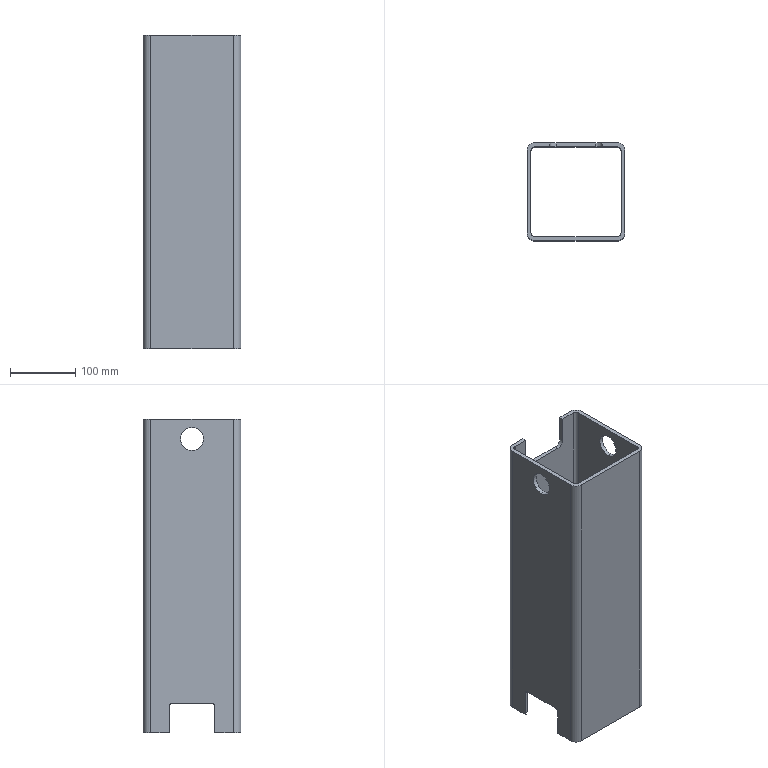Part | SolidWorks | features ICE 2, Attribute 1, Chamfer 1, Extrusion 1 | 1 solid | 48 faces | box 150 x 150 x 480 mm | volume 1538140 mm3 | plane 26 | cylinder 18 | cone 4 | commonest cylinder face diameters 10 x4 12 x4 24 x4 35 x4 20 x2
STEP:
#1=CARTESIAN_POINT('',(-75.,0.,227.5));
#2=VERTEX_POINT('',#1);
#3=CARTESIAN_POINT('',(-75.,0.,192.5));
#4=VERTEX_POINT('',#3);
#5=CARTESIAN_POINT('',(-75.,0.,210.));
#6=DIRECTION('',(1.,0.,0.));
#7=DIRECTION('',(0.,0.,-1.));
#8=AXIS2_PLACEMENT_3D('',#5,#6,#7);
#9=CIRCLE('',#8,17.5);
#10=EDGE_CURVE('',#2,#4,#9,.T.);
#11=ORIENTED_EDGE('',*,*,#10,.F.);
#12=CARTESIAN_POINT('',(-69.,0.,227.5));
#13=VERTEX_POINT('',#12);
#14=CARTESIAN_POINT('',(-75.,0.,227.5));
#15=DIRECTION('',(1.,0.,0.));
#16=VECTOR('',#15,1000.);
#17=LINE('',#14,#16);
#18=EDGE_CURVE('',#2,#13,#17,.T.);
#19=ORIENTED_EDGE('',*,*,#18,.T.);
#20=CARTESIAN_POINT('',(-69.,0.,192.5));
#21=VERTEX_POINT('',#20);
#22=CARTESIAN_POINT('',(-69.,0.,210.));
#23=DIRECTION('',(1.,0.,0.));
#24=DIRECTION('',(0.,0.,-1.));
#25=AXIS2_PLACEMENT_3D('',#22,#23,#24);
#26=CIRCLE('',#25,17.5);
#27=EDGE_CURVE('',#13,#21,#26,.T.);
#28=ORIENTED_EDGE('',*,*,#27,.T.);
#29=CARTESIAN_POINT('',(-75.,0.,192.5));
#30=DIRECTION('',(1.,0.,0.));
#31=VECTOR('',#30,1000.);
#32=LINE('',#29,#31);
#33=EDGE_CURVE('',#4,#21,#32,.T.);
#34=ORIENTED_EDGE('',*,*,#33,.F.);
#35=EDGE_LOOP('',(#11,#19,#28,#34));
#36=FACE_OUTER_BOUND('',#35,.T.);
#37=CARTESIAN_POINT('',(-75.,0.,210.));
#38=DIRECTION('',(1.,0.,0.));
#39=DIRECTION('',(0.,0.,-1.));
#40=AXIS2_PLACEMENT_3D('',#37,#38,#39);
#41=CYLINDRICAL_SURFACE('',#40,17.5);
#42=ADVANCED_FACE('',(#36),#41,.F.);
#43=CARTESIAN_POINT('',(69.,0.,192.5));
#44=VERTEX_POINT('',#43);
#45=CARTESIAN_POINT('',(69.,0.,227.5));
#46=VERTEX_POINT('',#45);
#47=CARTESIAN_POINT('',(69.,0.,210.));
#48=DIRECTION('',(-1.,0.,0.));
#49=DIRECTION('',(0.,0.,1.));
#50=AXIS2_PLACEMENT_3D('',#47,#48,#49);
#51=CIRCLE('',#50,17.5);
#52=EDGE_CURVE('',#44,#46,#51,.T.);
#53=ORIENTED_EDGE('',*,*,#52,.T.);
#54=CARTESIAN_POINT('',(75.,0.,227.5));
#55=VERTEX_POINT('',#54);
#56=CARTESIAN_POINT('',(-75.,0.,227.5));
#57=DIRECTION('',(1.,0.,0.));
#58=VECTOR('',#57,1000.);
#59=LINE('',#56,#58);
#60=EDGE_CURVE('',#46,#55,#59,.T.);
#61=ORIENTED_EDGE('',*,*,#60,.T.);
#62=CARTESIAN_POINT('',(75.,0.,192.5));
#63=VERTEX_POINT('',#62);
#64=CARTESIAN_POINT('',(75.,0.,210.));
#65=DIRECTION('',(1.,0.,0.));
#66=DIRECTION('',(0.,0.,-1.));
#67=AXIS2_PLACEMENT_3D('',#64,#65,#66);
#68=CIRCLE('',#67,17.5);
#69=EDGE_CURVE('',#55,#63,#68,.T.);
#70=ORIENTED_EDGE('',*,*,#69,.T.);
#71=CARTESIAN_POINT('',(-75.,0.,192.5));
#72=DIRECTION('',(1.,0.,0.));
#73=VECTOR('',#72,1000.);
#74=LINE('',#71,#73);
#75=EDGE_CURVE('',#44,#63,#74,.T.);
#76=ORIENTED_EDGE('',*,*,#75,.F.);
#77=EDGE_LOOP('',(#53,#61,#70,#76));
#78=FACE_OUTER_BOUND('',#77,.T.);
#79=CARTESIAN_POINT('',(-75.,0.,210.));
#80=DIRECTION('',(1.,0.,0.));
#81=DIRECTION('',(0.,0.,-1.));
#82=AXIS2_PLACEMENT_3D('',#79,#80,#81);
#83=CYLINDRICAL_SURFACE('',#82,17.5);
#84=ADVANCED_FACE('',(#78),#83,.F.);
#85=CARTESIAN_POINT('',(63.,-73.,-240.));
#86=VERTEX_POINT('',#85);
#87=CARTESIAN_POINT('',(73.,-63.,-240.));
#88=VERTEX_POINT('',#87);
#89=CARTESIAN_POINT('',(63.,-63.,-240.));
#90=DIRECTION('',(0.,0.,1.));
#91=DIRECTION('',(1.,0.,0.));
#92=AXIS2_PLACEMENT_3D('',#89,#90,#91);
#93=CIRCLE('',#92,10.);
#94=EDGE_CURVE('',#86,#88,#93,.T.);
#95=ORIENTED_EDGE('',*,*,#94,.T.);
#96=CARTESIAN_POINT('',(73.,-35.,-240.));
#97=VERTEX_POINT('',#96);
#98=CARTESIAN_POINT('',(73.,-35.,-240.));
#99=DIRECTION('',(0.,1.,0.));
#100=VECTOR('',#99,1000.);
#101=LINE('',#98,#100);
#102=EDGE_CURVE('',#88,#97,#101,.T.);
#103=ORIENTED_EDGE('',*,*,#102,.T.);
#104=CARTESIAN_POINT('',(75.,-35.,-240.));
#105=VERTEX_POINT('',#104);
#106=CARTESIAN_POINT('',(63.,-35.,-240.));
#107=DIRECTION('',(1.,0.,0.));
#108=VECTOR('',#107,1000.);
#109=LINE('',#106,#108);
#110=EDGE_CURVE('',#97,#105,#109,.T.);
#111=ORIENTED_EDGE('',*,*,#110,.T.);
#112=CARTESIAN_POINT('',(75.,-63.,-240.));
#113=VERTEX_POINT('',#112);
#114=CARTESIAN_POINT('',(75.,63.,-240.));
#115=DIRECTION('',(0.,1.,0.));
#116=VECTOR('',#115,1000.);
#117=LINE('',#114,#116);
#118=EDGE_CURVE('',#113,#105,#117,.T.);
#119=ORIENTED_EDGE('',*,*,#118,.F.);
#120=CARTESIAN_POINT('',(63.,-75.,-240.));
#121=VERTEX_POINT('',#120);
#122=CARTESIAN_POINT('',(63.,-63.,-240.));
#123=DIRECTION('',(0.,0.,1.));
#124=DIRECTION('',(1.,0.,0.));
#125=AXIS2_PLACEMENT_3D('',#122,#123,#124);
#126=CIRCLE('',#125,12.);
#127=EDGE_CURVE('',#121,#113,#126,.T.);
#128=ORIENTED_EDGE('',*,*,#127,.F.);
#129=CARTESIAN_POINT('',(-63.,-75.,-240.));
#130=VERTEX_POINT('',#129);
#131=CARTESIAN_POINT('',(-63.,-75.,-240.));
#132=DIRECTION('',(1.,0.,0.));
#133=VECTOR('',#132,1000.);
#134=LINE('',#131,#133);
#135=EDGE_CURVE('',#130,#121,#134,.T.);
#136=ORIENTED_EDGE('',*,*,#135,.F.);
#137=CARTESIAN_POINT('',(-75.,-63.,-240.));
#138=VERTEX_POINT('',#137);
#139=CARTESIAN_POINT('',(-63.,-63.,-240.));
#140=DIRECTION('',(0.,0.,1.));
#141=DIRECTION('',(1.,0.,0.));
#142=AXIS2_PLACEMENT_3D('',#139,#140,#141);
#143=CIRCLE('',#142,12.);
#144=EDGE_CURVE('',#138,#130,#143,.T.);
#145=ORIENTED_EDGE('',*,*,#144,.F.);
#146=CARTESIAN_POINT('',(-75.,-35.,-240.));
#147=VERTEX_POINT('',#146);
#148=CARTESIAN_POINT('',(-75.,-63.,-240.));
#149=DIRECTION('',(0.,-1.,0.));
#150=VECTOR('',#149,1000.);
#151=LINE('',#148,#150);
#152=EDGE_CURVE('',#147,#138,#151,.T.);
#153=ORIENTED_EDGE('',*,*,#152,.F.);
#154=CARTESIAN_POINT('',(-73.,-35.,-240.));
#155=VERTEX_POINT('',#154);
#156=CARTESIAN_POINT('',(63.,-35.,-240.));
#157=DIRECTION('',(1.,0.,0.));
#158=VECTOR('',#157,1000.);
#159=LINE('',#156,#158);
#160=EDGE_CURVE('',#147,#155,#159,.T.);
#161=ORIENTED_EDGE('',*,*,#160,.T.);
#162=CARTESIAN_POINT('',(-73.,-63.,-240.));
#163=VERTEX_POINT('',#162);
#164=CARTESIAN_POINT('',(-73.,-63.,-240.));
#165=DIRECTION('',(0.,-1.,0.));
#166=VECTOR('',#165,1000.);
#167=LINE('',#164,#166);
#168=EDGE_CURVE('',#155,#163,#167,.T.);
#169=ORIENTED_EDGE('',*,*,#168,.T.);
#170=CARTESIAN_POINT('',(-63.,-73.,-240.));
#171=VERTEX_POINT('',#170);
#172=CARTESIAN_POINT('',(-63.,-63.,-240.));
#173=DIRECTION('',(0.,0.,1.));
#174=DIRECTION('',(1.,0.,0.));
#175=AXIS2_PLACEMENT_3D('',#172,#173,#174);
#176=CIRCLE('',#175,10.);
#177=EDGE_CURVE('',#163,#171,#176,.T.);
#178=ORIENTED_EDGE('',*,*,#177,.T.);
#179=CARTESIAN_POINT('',(63.,-73.,-240.));
#180=DIRECTION('',(1.,0.,0.));
#181=VECTOR('',#180,1000.);
#182=LINE('',#179,#181);
#183=EDGE_CURVE('',#171,#86,#182,.T.);
#184=ORIENTED_EDGE('',*,*,#183,.T.);
#185=EDGE_LOOP('',(#95,#103,#111,#119,#128,#136,#145,#153,#161,#169,#178,#184));
#186=FACE_OUTER_BOUND('',#185,.T.);
#187=CARTESIAN_POINT('',(63.,63.,-240.));
#188=DIRECTION('',(0.,0.,1.));
#189=DIRECTION('',(1.,0.,0.));
#190=AXIS2_PLACEMENT_3D('',#187,#188,#189);
#191=PLANE('',#190);
#192=ADVANCED_FACE('',(#186),#191,.F.);
#193=CARTESIAN_POINT('',(63.,75.,240.));
#194=VERTEX_POINT('',#193);
#195=CARTESIAN_POINT('',(40.,75.,240.));
#196=VERTEX_POINT('',#195);
#197=CARTESIAN_POINT('',(63.,75.,240.));
#198=DIRECTION('',(-1.,0.,0.));
#199=VECTOR('',#198,1000.);
#200=LINE('',#197,#199);
#201=EDGE_CURVE('',#194,#196,#200,.T.);
#202=ORIENTED_EDGE('',*,*,#201,.T.);
#203=CARTESIAN_POINT('',(40.,69.,240.));
#204=VERTEX_POINT('',#203);
#205=CARTESIAN_POINT('',(40.,63.,240.));
#206=DIRECTION('',(0.,-1.,0.));
#207=VECTOR('',#206,1000.);
#208=LINE('',#205,#207);
#209=EDGE_CURVE('',#196,#204,#208,.T.);
#210=ORIENTED_EDGE('',*,*,#209,.T.);
#211=CARTESIAN_POINT('',(63.,69.,240.));
#212=VERTEX_POINT('',#211);
#213=CARTESIAN_POINT('',(63.,69.,240.));
#214=DIRECTION('',(-1.,0.,0.));
#215=VECTOR('',#214,1000.);
#216=LINE('',#213,#215);
#217=EDGE_CURVE('',#212,#204,#216,.T.);
#218=ORIENTED_EDGE('',*,*,#217,.F.);
#219=CARTESIAN_POINT('',(69.,63.,240.));
#220=VERTEX_POINT('',#219);
#221=CARTESIAN_POINT('',(63.,63.,240.));
#222=DIRECTION('',(0.,0.,1.));
#223=DIRECTION('',(1.,0.,0.));
#224=AXIS2_PLACEMENT_3D('',#221,#222,#223);
#225=CIRCLE('',#224,6.);
#226=EDGE_CURVE('',#220,#212,#225,.T.);
#227=ORIENTED_EDGE('',*,*,#226,.F.);
#228=CARTESIAN_POINT('',(69.,-63.,240.));
#229=VERTEX_POINT('',#228);
#230=CARTESIAN_POINT('',(69.,63.,240.));
#231=DIRECTION('',(0.,1.,0.));
#232=VECTOR('',#231,1000.);
#233=LINE('',#230,#232);
#234=EDGE_CURVE('',#229,#220,#233,.T.);
#235=ORIENTED_EDGE('',*,*,#234,.F.);
#236=CARTESIAN_POINT('',(63.,-69.,240.));
#237=VERTEX_POINT('',#236);
#238=CARTESIAN_POINT('',(63.,-63.,240.));
#239=DIRECTION('',(0.,0.,1.));
#240=DIRECTION('',(1.,0.,0.));
#241=AXIS2_PLACEMENT_3D('',#238,#239,#240);
#242=CIRCLE('',#241,6.);
#243=EDGE_CURVE('',#237,#229,#242,.T.);
#244=ORIENTED_EDGE('',*,*,#243,.F.);
#245=CARTESIAN_POINT('',(-63.,-69.,240.));
#246=VERTEX_POINT('',#245);
#247=CARTESIAN_POINT('',(-63.,-69.,240.));
#248=DIRECTION('',(1.,0.,0.));
#249=VECTOR('',#248,1000.);
#250=LINE('',#247,#249);
#251=EDGE_CURVE('',#246,#237,#250,.T.);
#252=ORIENTED_EDGE('',*,*,#251,.F.);
#253=CARTESIAN_POINT('',(-69.,-63.,240.));
#254=VERTEX_POINT('',#253);
#255=CARTESIAN_POINT('',(-63.,-63.,240.));
#256=DIRECTION('',(0.,0.,1.));
#257=DIRECTION('',(1.,0.,0.));
#258=AXIS2_PLACEMENT_3D('',#255,#256,#257);
#259=CIRCLE('',#258,6.);
#260=EDGE_CURVE('',#254,#246,#259,.T.);
#261=ORIENTED_EDGE('',*,*,#260,.F.);
#262=CARTESIAN_POINT('',(-69.,63.,240.));
#263=VERTEX_POINT('',#262);
#264=CARTESIAN_POINT('',(-69.,-63.,240.));
#265=DIRECTION('',(0.,-1.,0.));
#266=VECTOR('',#265,1000.);
#267=LINE('',#264,#266);
#268=EDGE_CURVE('',#263,#254,#267,.T.);
#269=ORIENTED_EDGE('',*,*,#268,.F.);
#270=CARTESIAN_POINT('',(-63.,69.,240.));
#271=VERTEX_POINT('',#270);
#272=CARTESIAN_POINT('',(-63.,63.,240.));
#273=DIRECTION('',(0.,0.,1.));
#274=DIRECTION('',(1.,0.,0.));
#275=AXIS2_PLACEMENT_3D('',#272,#273,#274);
#276=CIRCLE('',#275,6.);
#277=EDGE_CURVE('',#271,#263,#276,.T.);
#278=ORIENTED_EDGE('',*,*,#277,.F.);
#279=CARTESIAN_POINT('',(-40.,69.,240.));
#280=VERTEX_POINT('',#279);
#281=CARTESIAN_POINT('',(63.,69.,240.));
#282=DIRECTION('',(-1.,0.,0.));
#283=VECTOR('',#282,1000.);
#284=LINE('',#281,#283);
#285=EDGE_CURVE('',#280,#271,#284,.T.);
#286=ORIENTED_EDGE('',*,*,#285,.F.);
#287=CARTESIAN_POINT('',(-40.,75.,240.));
#288=VERTEX_POINT('',#287);
#289=CARTESIAN_POINT('',(-40.,63.,240.));
#290=DIRECTION('',(0.,1.,0.));
#291=VECTOR('',#290,1000.);
#292=LINE('',#289,#291);
#293=EDGE_CURVE('',#280,#288,#292,.T.);
#294=ORIENTED_EDGE('',*,*,#293,.T.);
#295=CARTESIAN_POINT('',(-63.,75.,240.));
#296=VERTEX_POINT('',#295);
#297=CARTESIAN_POINT('',(63.,75.,240.));
#298=DIRECTION('',(-1.,0.,0.));
#299=VECTOR('',#298,1000.);
#300=LINE('',#297,#299);
#301=EDGE_CURVE('',#288,#296,#300,.T.);
#302=ORIENTED_EDGE('',*,*,#301,.T.);
#303=CARTESIAN_POINT('',(-75.,63.,240.));
#304=VERTEX_POINT('',#303);
#305=CARTESIAN_POINT('',(-63.,63.,240.));
#306=DIRECTION('',(0.,0.,1.));
#307=DIRECTION('',(1.,0.,0.));
#308=AXIS2_PLACEMENT_3D('',#305,#306,#307);
#309=CIRCLE('',#308,12.);
#310=EDGE_CURVE('',#296,#304,#309,.T.);
#311=ORIENTED_EDGE('',*,*,#310,.T.);
#312=CARTESIAN_POINT('',(-75.,-63.,240.));
#313=VERTEX_POINT('',#312);
#314=CARTESIAN_POINT('',(-75.,-63.,240.));
#315=DIRECTION('',(0.,-1.,0.));
#316=VECTOR('',#315,1000.);
#317=LINE('',#314,#316);
#318=EDGE_CURVE('',#304,#313,#317,.T.);
#319=ORIENTED_EDGE('',*,*,#318,.T.);
#320=CARTESIAN_POINT('',(-63.,-75.,240.));
#321=VERTEX_POINT('',#320);
#322=CARTESIAN_POINT('',(-63.,-63.,240.));
#323=DIRECTION('',(0.,0.,1.));
#324=DIRECTION('',(1.,0.,0.));
#325=AXIS2_PLACEMENT_3D('',#322,#323,#324);
#326=CIRCLE('',#325,12.);
#327=EDGE_CURVE('',#313,#321,#326,.T.);
#328=ORIENTED_EDGE('',*,*,#327,.T.);
#329=CARTESIAN_POINT('',(63.,-75.,240.));
#330=VERTEX_POINT('',#329);
#331=CARTESIAN_POINT('',(-63.,-75.,240.));
#332=DIRECTION('',(1.,0.,0.));
#333=VECTOR('',#332,1000.);
#334=LINE('',#331,#333);
#335=EDGE_CURVE('',#321,#330,#334,.T.);
#336=ORIENTED_EDGE('',*,*,#335,.T.);
#337=CARTESIAN_POINT('',(75.,-63.,240.));
#338=VERTEX_POINT('',#337);
#339=CARTESIAN_POINT('',(63.,-63.,240.));
#340=DIRECTION('',(0.,0.,1.));
#341=DIRECTION('',(1.,0.,0.));
#342=AXIS2_PLACEMENT_3D('',#339,#340,#341);
#343=CIRCLE('',#342,12.);
#344=EDGE_CURVE('',#330,#338,#343,.T.);
#345=ORIENTED_EDGE('',*,*,#344,.T.);
#346=CARTESIAN_POINT('',(75.,63.,240.));
#347=VERTEX_POINT('',#346);
#348=CARTESIAN_POINT('',(75.,63.,240.));
#349=DIRECTION('',(0.,1.,0.));
#350=VECTOR('',#349,1000.);
#351=LINE('',#348,#350);
#352=EDGE_CURVE('',#338,#347,#351,.T.);
#353=ORIENTED_EDGE('',*,*,#352,.T.);
#354=CARTESIAN_POINT('',(63.,63.,240.));
#355=DIRECTION('',(0.,0.,1.));
#356=DIRECTION('',(1.,0.,0.));
#357=AXIS2_PLACEMENT_3D('',#354,#355,#356);
#358=CIRCLE('',#357,12.);
#359=EDGE_CURVE('',#347,#194,#358,.T.);
#360=ORIENTED_EDGE('',*,*,#359,.T.);
#361=EDGE_LOOP('',(#202,#210,#218,#227,#235,#244,#252,#261,#269,#278,#286,#294,#302,#311,#319,#328,#336,#345,#353,#360));
#362=FACE_OUTER_BOUND('',#361,.T.);
#363=CARTESIAN_POINT('',(63.,63.,240.));
#364=DIRECTION('',(0.,0.,1.));
#365=DIRECTION('',(1.,0.,0.));
#366=AXIS2_PLACEMENT_3D('',#363,#364,#365);
#367=PLANE('',#366);
#368=ADVANCED_FACE('',(#362),#367,.T.);
#369=CARTESIAN_POINT('',(40.,75.,200.));
#370=VERTEX_POINT('',#369);
#371=CARTESIAN_POINT('',(40.,75.,290.));
#372=DIRECTION('',(0.,0.,-1.));
#373=VECTOR('',#372,1000.);
#374=LINE('',#371,#373);
#375=EDGE_CURVE('',#196,#370,#374,.T.);
#376=ORIENTED_EDGE('',*,*,#375,.F.);
#377=ORIENTED_EDGE('',*,*,#201,.F.);
#378=CARTESIAN_POINT('',(63.,75.,-240.));
#379=VERTEX_POINT('',#378);
#380=CARTESIAN_POINT('',(63.,75.,240.));
#381=DIRECTION('',(0.,0.,-1.));
#382=VECTOR('',#381,1000.);
#383=LINE('',#380,#382);
#384=EDGE_CURVE('',#194,#379,#383,.T.);
#385=ORIENTED_EDGE('',*,*,#384,.T.);
#386=CARTESIAN_POINT('',(-63.,75.,-240.));
#387=VERTEX_POINT('',#386);
#388=CARTESIAN_POINT('',(63.,75.,-240.));
#389=DIRECTION('',(-1.,0.,0.));
#390=VECTOR('',#389,1000.);
#391=LINE('',#388,#390);
#392=EDGE_CURVE('',#379,#387,#391,.T.);
#393=ORIENTED_EDGE('',*,*,#392,.T.);
#394=CARTESIAN_POINT('',(-63.,75.,240.));
#395=DIRECTION('',(0.,0.,-1.));
#396=VECTOR('',#395,1000.);
#397=LINE('',#394,#396);
#398=EDGE_CURVE('',#296,#387,#397,.T.);
#399=ORIENTED_EDGE('',*,*,#398,.F.);
#400=ORIENTED_EDGE('',*,*,#301,.F.);
#401=CARTESIAN_POINT('',(-40.,75.,200.));
#402=VERTEX_POINT('',#401);
#403=CARTESIAN_POINT('',(-40.,75.,290.));
#404=DIRECTION('',(0.,0.,1.));
#405=VECTOR('',#404,1000.);
#406=LINE('',#403,#405);
#407=EDGE_CURVE('',#402,#288,#406,.T.);
#408=ORIENTED_EDGE('',*,*,#407,.F.);
#409=CARTESIAN_POINT('',(-30.,75.,190.));
#410=VERTEX_POINT('',#409);
#411=CARTESIAN_POINT('',(-30.,75.,200.));
#412=DIRECTION('',(0.,1.,0.));
#413=DIRECTION('',(0.,0.,1.));
#414=AXIS2_PLACEMENT_3D('',#411,#412,#413);
#415=CIRCLE('',#414,10.);
#416=EDGE_CURVE('',#410,#402,#415,.T.);
#417=ORIENTED_EDGE('',*,*,#416,.F.);
#418=CARTESIAN_POINT('',(30.,75.,190.));
#419=VERTEX_POINT('',#418);
#420=CARTESIAN_POINT('',(30.,75.,190.));
#421=DIRECTION('',(-1.,0.,0.));
#422=VECTOR('',#421,1000.);
#423=LINE('',#420,#422);
#424=EDGE_CURVE('',#419,#410,#423,.T.);
#425=ORIENTED_EDGE('',*,*,#424,.F.);
#426=CARTESIAN_POINT('',(30.,75.,200.));
#427=DIRECTION('',(0.,1.,0.));
#428=DIRECTION('',(0.,0.,1.));
#429=AXIS2_PLACEMENT_3D('',#426,#427,#428);
#430=CIRCLE('',#429,10.);
#431=EDGE_CURVE('',#370,#419,#430,.T.);
#432=ORIENTED_EDGE('',*,*,#431,.F.);
#433=EDGE_LOOP('',(#376,#377,#385,#393,#399,#400,#408,#417,#425,#432));
#434=FACE_OUTER_BOUND('',#433,.T.);
#435=CARTESIAN_POINT('',(63.,75.,240.));
#436=DIRECTION('',(0.,-1.,0.));
#437=DIRECTION('',(0.,0.,-1.));
#438=AXIS2_PLACEMENT_3D('',#435,#436,#437);
#439=PLANE('',#438);
#440=ADVANCED_FACE('',(#434),#439,.F.);
#441=CARTESIAN_POINT('',(-63.,69.,-236.));
#442=VERTEX_POINT('',#441);
#443=CARTESIAN_POINT('',(-63.,69.,240.));
#444=DIRECTION('',(0.,0.,-1.));
#445=VECTOR('',#444,1000.);
#446=LINE('',#443,#445);
#447=EDGE_CURVE('',#271,#442,#446,.T.);
#448=ORIENTED_EDGE('',*,*,#447,.T.);
#449=CARTESIAN_POINT('',(63.,69.,-236.));
#450=VERTEX_POINT('',#449);
#451=CARTESIAN_POINT('',(63.,69.,-236.));
#452=DIRECTION('',(1.,0.,0.));
#453=VECTOR('',#452,1000.);
#454=LINE('',#451,#453);
#455=EDGE_CURVE('',#442,#450,#454,.T.);
#456=ORIENTED_EDGE('',*,*,#455,.T.);
#457=CARTESIAN_POINT('',(63.,69.,240.));
#458=DIRECTION('',(0.,0.,-1.));
#459=VECTOR('',#458,1000.);
#460=LINE('',#457,#459);
#461=EDGE_CURVE('',#212,#450,#460,.T.);
#462=ORIENTED_EDGE('',*,*,#461,.F.);
#463=ORIENTED_EDGE('',*,*,#217,.T.);
#464=CARTESIAN_POINT('',(40.,69.,200.));
#465=VERTEX_POINT('',#464);
#466=CARTESIAN_POINT('',(40.,69.,240.));
#467=DIRECTION('',(0.,0.,-1.));
#468=VECTOR('',#467,1000.);
#469=LINE('',#466,#468);
#470=EDGE_CURVE('',#204,#465,#469,.T.);
#471=ORIENTED_EDGE('',*,*,#470,.T.);
#472=CARTESIAN_POINT('',(30.,69.,190.));
#473=VERTEX_POINT('',#472);
#474=CARTESIAN_POINT('',(30.,69.,200.));
#475=DIRECTION('',(0.,1.,0.));
#476=DIRECTION('',(0.,0.,-1.));
#477=AXIS2_PLACEMENT_3D('',#474,#475,#476);
#478=CIRCLE('',#477,10.);
#479=EDGE_CURVE('',#465,#473,#478,.T.);
#480=ORIENTED_EDGE('',*,*,#479,.T.);
#481=CARTESIAN_POINT('',(-30.,69.,190.));
#482=VERTEX_POINT('',#481);
#483=CARTESIAN_POINT('',(63.,69.,190.));
#484=DIRECTION('',(-1.,0.,0.));
#485=VECTOR('',#484,1000.);
#486=LINE('',#483,#485);
#487=EDGE_CURVE('',#473,#482,#486,.T.);
#488=ORIENTED_EDGE('',*,*,#487,.T.);
#489=CARTESIAN_POINT('',(-40.,69.,200.));
#490=VERTEX_POINT('',#489);
#491=CARTESIAN_POINT('',(-30.,69.,200.));
#492=DIRECTION('',(0.,1.,0.));
#493=DIRECTION('',(0.,0.,-1.));
#494=AXIS2_PLACEMENT_3D('',#491,#492,#493);
#495=CIRCLE('',#494,10.);
#496=EDGE_CURVE('',#482,#490,#495,.T.);
#497=ORIENTED_EDGE('',*,*,#496,.T.);
#498=CARTESIAN_POINT('',(-40.,69.,240.));
#499=DIRECTION('',(0.,0.,1.));
#500=VECTOR('',#499,1000.);
#501=LINE('',#498,#500);
#502=EDGE_CURVE('',#490,#280,#501,.T.);
#503=ORIENTED_EDGE('',*,*,#502,.T.);
#504=ORIENTED_EDGE('',*,*,#285,.T.);
#505=EDGE_LOOP('',(#448,#456,#462,#463,#471,#480,#488,#497,#503,#504));
#506=FACE_OUTER_BOUND('',#505,.T.);
#507=CARTESIAN_POINT('',(63.,69.,240.));
#508=DIRECTION('',(0.,-1.,0.));
#509=DIRECTION('',(0.,0.,-1.));
#510=AXIS2_PLACEMENT_3D('',#507,#508,#509);
#511=PLANE('',#510);
#512=ADVANCED_FACE('',(#506),#511,.T.);
#513=CARTESIAN_POINT('',(75.,35.,-240.));
#514=VERTEX_POINT('',#513);
#515=CARTESIAN_POINT('',(73.,35.,-240.));
#516=VERTEX_POINT('',#515);
#517=CARTESIAN_POINT('',(63.,35.,-240.));
#518=DIRECTION('',(-1.,0.,0.));
#519=VECTOR('',#518,1000.);
#520=LINE('',#517,#519);
#521=EDGE_CURVE('',#514,#516,#520,.T.);
#522=ORIENTED_EDGE('',*,*,#521,.T.);
#523=CARTESIAN_POINT('',(73.,63.,-240.));
#524=VERTEX_POINT('',#523);
#525=CARTESIAN_POINT('',(73.,63.,-240.));
#526=DIRECTION('',(0.,1.,0.));
#527=VECTOR('',#526,1000.);
#528=LINE('',#525,#527);
#529=EDGE_CURVE('',#516,#524,#528,.T.);
#530=ORIENTED_EDGE('',*,*,#529,.T.);
#531=CARTESIAN_POINT('',(63.,73.,-240.));
#532=VERTEX_POINT('',#531);
#533=CARTESIAN_POINT('',(63.,63.,-240.));
#534=DIRECTION('',(0.,0.,1.));
#535=DIRECTION('',(1.,0.,0.));
#536=AXIS2_PLACEMENT_3D('',#533,#534,#535);
#537=CIRCLE('',#536,10.);
#538=EDGE_CURVE('',#524,#532,#537,.T.);
#539=ORIENTED_EDGE('',*,*,#538,.T.);
#540=CARTESIAN_POINT('',(-63.,73.,-240.));
#541=VERTEX_POINT('',#540);
#542=CARTESIAN_POINT('',(-63.,73.,-240.));
#543=DIRECTION('',(-1.,0.,0.));
#544=VECTOR('',#543,1000.);
#545=LINE('',#542,#544);
#546=EDGE_CURVE('',#532,#541,#545,.T.);
#547=ORIENTED_EDGE('',*,*,#546,.T.);
#548=CARTESIAN_POINT('',(-73.,63.,-240.));
#549=VERTEX_POINT('',#548);
#550=CARTESIAN_POINT('',(-63.,63.,-240.));
#551=DIRECTION('',(0.,0.,1.));
#552=DIRECTION('',(1.,0.,0.));
#553=AXIS2_PLACEMENT_3D('',#550,#551,#552);
#554=CIRCLE('',#553,10.);
#555=EDGE_CURVE('',#541,#549,#554,.T.);
#556=ORIENTED_EDGE('',*,*,#555,.T.);
#557=CARTESIAN_POINT('',(-73.,35.,-240.));
#558=VERTEX_POINT('',#557);
#559=CARTESIAN_POINT('',(-73.,35.,-240.));
#560=DIRECTION('',(0.,-1.,0.));
#561=VECTOR('',#560,1000.);
#562=LINE('',#559,#561);
#563=EDGE_CURVE('',#549,#558,#562,.T.);
#564=ORIENTED_EDGE('',*,*,#563,.T.);
#565=CARTESIAN_POINT('',(-75.,35.,-240.));
#566=VERTEX_POINT('',#565);
#567=CARTESIAN_POINT('',(63.,35.,-240.));
#568=DIRECTION('',(-1.,0.,0.));
#569=VECTOR('',#568,1000.);
#570=LINE('',#567,#569);
#571=EDGE_CURVE('',#558,#566,#570,.T.);
#572=ORIENTED_EDGE('',*,*,#571,.T.);
#573=CARTESIAN_POINT('',(-75.,63.,-240.));
#574=VERTEX_POINT('',#573);
#575=CARTESIAN_POINT('',(-75.,-63.,-240.));
#576=DIRECTION('',(0.,-1.,0.));
#577=VECTOR('',#576,1000.);
#578=LINE('',#575,#577);
#579=EDGE_CURVE('',#574,#566,#578,.T.);
#580=ORIENTED_EDGE('',*,*,#579,.F.);
#581=CARTESIAN_POINT('',(-63.,63.,-240.));
#582=DIRECTION('',(0.,0.,1.));
#583=DIRECTION('',(1.,0.,0.));
#584=AXIS2_PLACEMENT_3D('',#581,#582,#583);
#585=CIRCLE('',#584,12.);
#586=EDGE_CURVE('',#387,#574,#585,.T.);
#587=ORIENTED_EDGE('',*,*,#586,.F.);
#588=ORIENTED_EDGE('',*,*,#392,.F.);
#589=CARTESIAN_POINT('',(75.,63.,-240.));
#590=VERTEX_POINT('',#589);
#591=CARTESIAN_POINT('',(63.,63.,-240.));
#592=DIRECTION('',(0.,0.,1.));
#593=DIRECTION('',(1.,0.,0.));
#594=AXIS2_PLACEMENT_3D('',#591,#592,#593);
#595=CIRCLE('',#594,12.);
#596=EDGE_CURVE('',#590,#379,#595,.T.);
#597=ORIENTED_EDGE('',*,*,#596,.F.);
#598=CARTESIAN_POINT('',(75.,63.,-240.));
#599=DIRECTION('',(0.,1.,0.));
#600=VECTOR('',#599,1000.);
#601=LINE('',#598,#600);
#602=EDGE_CURVE('',#514,#590,#601,.T.);
#603=ORIENTED_EDGE('',*,*,#602,.F.);
#604=EDGE_LOOP('',(#522,#530,#539,#547,#556,#564,#572,#580,#587,#588,#597,#603));
#605=FACE_OUTER_BOUND('',#604,.T.);
#606=CARTESIAN_POINT('',(63.,63.,-240.));
#607=DIRECTION('',(0.,0.,1.));
#608=DIRECTION('',(1.,0.,0.));
#609=AXIS2_PLACEMENT_3D('',#606,#607,#608);
#610=PLANE('',#609);
#611=ADVANCED_FACE('',(#605),#610,.F.);
#612=ORIENTED_EDGE('',*,*,#596,.T.);
#613=ORIENTED_EDGE('',*,*,#384,.F.);
#614=ORIENTED_EDGE('',*,*,#359,.F.);
#615=CARTESIAN_POINT('',(75.,63.,240.));
#616=DIRECTION('',(0.,0.,-1.));
#617=VECTOR('',#616,1000.);
#618=LINE('',#615,#617);
#619=EDGE_CURVE('',#347,#590,#618,.T.);
#620=ORIENTED_EDGE('',*,*,#619,.T.);
#621=EDGE_LOOP('',(#612,#613,#614,#620));
#622=FACE_OUTER_BOUND('',#621,.T.);
#623=CARTESIAN_POINT('',(63.,63.,240.));
#624=DIRECTION('',(0.,0.,-1.));
#625=DIRECTION('',(-1.,0.,0.));
#626=AXIS2_PLACEMENT_3D('',#623,#624,#625);
#627=CYLINDRICAL_SURFACE('',#626,12.);
#628=ADVANCED_FACE('',(#622),#627,.T.);
#629=ORIENTED_EDGE('',*,*,#586,.T.);
#630=CARTESIAN_POINT('',(-75.,63.,240.));
#631=DIRECTION('',(0.,0.,-1.));
#632=VECTOR('',#631,1000.);
#633=LINE('',#630,#632);
#634=EDGE_CURVE('',#304,#574,#633,.T.);
#635=ORIENTED_EDGE('',*,*,#634,.F.);
#636=ORIENTED_EDGE('',*,*,#310,.F.);
#637=ORIENTED_EDGE('',*,*,#398,.T.);
#638=EDGE_LOOP('',(#629,#635,#636,#637));
#639=FACE_OUTER_BOUND('',#638,.T.);
#640=CARTESIAN_POINT('',(-63.,63.,240.));
#641=DIRECTION('',(0.,0.,-1.));
#642=DIRECTION('',(-1.,0.,0.));
#643=AXIS2_PLACEMENT_3D('',#640,#641,#642);
#644=CYLINDRICAL_SURFACE('',#643,12.);
#645=ADVANCED_FACE('',(#639),#644,.T.);
#646=CARTESIAN_POINT('',(-75.,0.,210.));
#647=DIRECTION('',(1.,0.,0.));
#648=DIRECTION('',(0.,0.,-1.));
#649=AXIS2_PLACEMENT_3D('',#646,#647,#648);
#650=CIRCLE('',#649,17.5);
#651=EDGE_CURVE('',#4,#2,#650,.T.);
#652=ORIENTED_EDGE('',*,*,#651,.T.);
#653=ORIENTED_EDGE('',*,*,#10,.T.);
#654=EDGE_LOOP('',(#652,#653));
#655=FACE_BOUND('',#654,.T.);
#656=CARTESIAN_POINT('',(-75.,-30.,-195.));
#657=VERTEX_POINT('',#656);
#658=CARTESIAN_POINT('',(-75.,-35.,-200.));
#659=VERTEX_POINT('',#658);
#660=CARTESIAN_POINT('',(-75.,-30.,-200.));
#661=DIRECTION('',(1.,0.,0.));
#662=DIRECTION('',(0.,0.,-1.));
#663=AXIS2_PLACEMENT_3D('',#660,#661,#662);
#664=CIRCLE('',#663,5.);
#665=EDGE_CURVE('',#657,#659,#664,.T.);
#666=ORIENTED_EDGE('',*,*,#665,.T.);
#667=CARTESIAN_POINT('',(-75.,-35.,-200.));
#668=DIRECTION('',(0.,0.,-1.));
#669=VECTOR('',#668,1000.);
#670=LINE('',#667,#669);
#671=EDGE_CURVE('',#659,#147,#670,.T.);
#672=ORIENTED_EDGE('',*,*,#671,.T.);
#673=ORIENTED_EDGE('',*,*,#152,.T.);
#674=CARTESIAN_POINT('',(-75.,-63.,240.));
#675=DIRECTION('',(0.,0.,-1.));
#676=VECTOR('',#675,1000.);
#677=LINE('',#674,#676);
#678=EDGE_CURVE('',#313,#138,#677,.T.);
#679=ORIENTED_EDGE('',*,*,#678,.F.);
#680=ORIENTED_EDGE('',*,*,#318,.F.);
#681=ORIENTED_EDGE('',*,*,#634,.T.);
#682=ORIENTED_EDGE('',*,*,#579,.T.);
#683=CARTESIAN_POINT('',(-75.,35.,-200.));
#684=VERTEX_POINT('',#683);
#685=CARTESIAN_POINT('',(-75.,35.,-200.));
#686=DIRECTION('',(0.,0.,1.));
#687=VECTOR('',#686,1000.);
#688=LINE('',#685,#687);
#689=EDGE_CURVE('',#566,#684,#688,.T.);
#690=ORIENTED_EDGE('',*,*,#689,.T.);
#691=CARTESIAN_POINT('',(-75.,30.,-195.));
#692=VERTEX_POINT('',#691);
#693=CARTESIAN_POINT('',(-75.,30.,-200.));
#694=DIRECTION('',(1.,0.,0.));
#695=DIRECTION('',(0.,0.,-1.));
#696=AXIS2_PLACEMENT_3D('',#693,#694,#695);
#697=CIRCLE('',#696,5.);
#698=EDGE_CURVE('',#684,#692,#697,.T.);
#699=ORIENTED_EDGE('',*,*,#698,.T.);
#700=CARTESIAN_POINT('',(-75.,30.,-195.));
#701=DIRECTION('',(0.,-1.,0.));
#702=VECTOR('',#701,1000.);
#703=LINE('',#700,#702);
#704=EDGE_CURVE('',#692,#657,#703,.T.);
#705=ORIENTED_EDGE('',*,*,#704,.T.);
#706=EDGE_LOOP('',(#666,#672,#673,#679,#680,#681,#682,#690,#699,#705));
#707=FACE_OUTER_BOUND('',#706,.T.);
#708=CARTESIAN_POINT('',(-75.,-63.,240.));
#709=DIRECTION('',(1.,0.,0.));
#710=DIRECTION('',(0.,0.,-1.));
#711=AXIS2_PLACEMENT_3D('',#708,#709,#710);
#712=PLANE('',#711);
#713=ADVANCED_FACE('',(#655,#707),#712,.F.);
#714=ORIENTED_EDGE('',*,*,#144,.T.);
#715=CARTESIAN_POINT('',(-63.,-75.,240.));
#716=DIRECTION('',(0.,0.,-1.));
#717=VECTOR('',#716,1000.);
#718=LINE('',#715,#717);
#719=EDGE_CURVE('',#321,#130,#718,.T.);
#720=ORIENTED_EDGE('',*,*,#719,.F.);
#721=ORIENTED_EDGE('',*,*,#327,.F.);
#722=ORIENTED_EDGE('',*,*,#678,.T.);
#723=EDGE_LOOP('',(#714,#720,#721,#722));
#724=FACE_OUTER_BOUND('',#723,.T.);
#725=CARTESIAN_POINT('',(-63.,-63.,240.));
#726=DIRECTION('',(0.,0.,-1.));
#727=DIRECTION('',(-1.,0.,0.));
#728=AXIS2_PLACEMENT_3D('',#725,#726,#727);
#729=CYLINDRICAL_SURFACE('',#728,12.);
#730=ADVANCED_FACE('',(#724),#729,.T.);
#731=ORIENTED_EDGE('',*,*,#135,.T.);
#732=CARTESIAN_POINT('',(63.,-75.,240.));
#733=DIRECTION('',(0.,0.,-1.));
#734=VECTOR('',#733,1000.);
#735=LINE('',#732,#734);
#736=EDGE_CURVE('',#330,#121,#735,.T.);
#737=ORIENTED_EDGE('',*,*,#736,.F.);
#738=ORIENTED_EDGE('',*,*,#335,.F.);
#739=ORIENTED_EDGE('',*,*,#719,.T.);
#740=EDGE_LOOP('',(#731,#737,#738,#739));
#741=FACE_OUTER_BOUND('',#740,.T.);
#742=CARTESIAN_POINT('',(-63.,-75.,240.));
#743=DIRECTION('',(0.,1.,0.));
#744=DIRECTION('',(0.,0.,1.));
#745=AXIS2_PLACEMENT_3D('',#742,#743,#744);
#746=PLANE('',#745);
#747=ADVANCED_FACE('',(#741),#746,.F.);
#748=ORIENTED_EDGE('',*,*,#127,.T.);
#749=CARTESIAN_POINT('',(75.,-63.,240.));
#750=DIRECTION('',(0.,0.,-1.));
#751=VECTOR('',#750,1000.);
#752=LINE('',#749,#751);
#753=EDGE_CURVE('',#338,#113,#752,.T.);
#754=ORIENTED_EDGE('',*,*,#753,.F.);
#755=ORIENTED_EDGE('',*,*,#344,.F.);
#756=ORIENTED_EDGE('',*,*,#736,.T.);
#757=EDGE_LOOP('',(#748,#754,#755,#756));
#758=FACE_OUTER_BOUND('',#757,.T.);
#759=CARTESIAN_POINT('',(63.,-63.,240.));
#760=DIRECTION('',(0.,0.,-1.));
#761=DIRECTION('',(-1.,0.,0.));
#762=AXIS2_PLACEMENT_3D('',#759,#760,#761);
#763=CYLINDRICAL_SURFACE('',#762,12.);
#764=ADVANCED_FACE('',(#758),#763,.T.);
#765=CARTESIAN_POINT('',(75.,0.,210.));
#766=DIRECTION('',(1.,0.,0.));
#767=DIRECTION('',(0.,0.,-1.));
#768=AXIS2_PLACEMENT_3D('',#765,#766,#767);
#769=CIRCLE('',#768,17.5);
#770=EDGE_CURVE('',#63,#55,#769,.T.);
#771=ORIENTED_EDGE('',*,*,#770,.F.);
#772=ORIENTED_EDGE('',*,*,#69,.F.);
#773=EDGE_LOOP('',(#771,#772));
#774=FACE_BOUND('',#773,.T.);
#775=ORIENTED_EDGE('',*,*,#118,.T.);
#776=CARTESIAN_POINT('',(75.,-35.,-200.));
#777=VERTEX_POINT('',#776);
#778=CARTESIAN_POINT('',(75.,-35.,-200.));
#779=DIRECTION('',(0.,0.,-1.));
#780=VECTOR('',#779,1000.);
#781=LINE('',#778,#780);
#782=EDGE_CURVE('',#777,#105,#781,.T.);
#783=ORIENTED_EDGE('',*,*,#782,.F.);
#784=CARTESIAN_POINT('',(75.,-30.,-195.));
#785=VERTEX_POINT('',#784);
#786=CARTESIAN_POINT('',(75.,-30.,-200.));
#787=DIRECTION('',(1.,0.,0.));
#788=DIRECTION('',(0.,0.,-1.));
#789=AXIS2_PLACEMENT_3D('',#786,#787,#788);
#790=CIRCLE('',#789,5.);
#791=EDGE_CURVE('',#785,#777,#790,.T.);
#792=ORIENTED_EDGE('',*,*,#791,.F.);
#793=CARTESIAN_POINT('',(75.,30.,-195.));
#794=VERTEX_POINT('',#793);
#795=CARTESIAN_POINT('',(75.,30.,-195.));
#796=DIRECTION('',(0.,-1.,0.));
#797=VECTOR('',#796,1000.);
#798=LINE('',#795,#797);
#799=EDGE_CURVE('',#794,#785,#798,.T.);
#800=ORIENTED_EDGE('',*,*,#799,.F.);
#801=CARTESIAN_POINT('',(75.,35.,-200.));
#802=VERTEX_POINT('',#801);
#803=CARTESIAN_POINT('',(75.,30.,-200.));
#804=DIRECTION('',(1.,0.,0.));
#805=DIRECTION('',(0.,0.,-1.));
#806=AXIS2_PLACEMENT_3D('',#803,#804,#805);
#807=CIRCLE('',#806,5.);
#808=EDGE_CURVE('',#802,#794,#807,.T.);
#809=ORIENTED_EDGE('',*,*,#808,.F.);
#810=CARTESIAN_POINT('',(75.,35.,-200.));
#811=DIRECTION('',(0.,0.,1.));
#812=VECTOR('',#811,1000.);
#813=LINE('',#810,#812);
#814=EDGE_CURVE('',#514,#802,#813,.T.);
#815=ORIENTED_EDGE('',*,*,#814,.F.);
#816=ORIENTED_EDGE('',*,*,#602,.T.);
#817=ORIENTED_EDGE('',*,*,#619,.F.);
#818=ORIENTED_EDGE('',*,*,#352,.F.);
#819=ORIENTED_EDGE('',*,*,#753,.T.);
#820=EDGE_LOOP('',(#775,#783,#792,#800,#809,#815,#816,#817,#818,#819));
#821=FACE_OUTER_BOUND('',#820,.T.);
#822=CARTESIAN_POINT('',(75.,63.,240.));
#823=DIRECTION('',(-1.,0.,0.));
#824=DIRECTION('',(0.,0.,1.));
#825=AXIS2_PLACEMENT_3D('',#822,#823,#824);
#826=PLANE('',#825);
#827=ADVANCED_FACE('',(#774,#821),#826,.F.);
#828=CARTESIAN_POINT('',(-69.,63.,-236.));
#829=VERTEX_POINT('',#828);
#830=CARTESIAN_POINT('',(-69.,63.,240.));
#831=DIRECTION('',(0.,0.,-1.));
#832=VECTOR('',#831,1000.);
#833=LINE('',#830,#832);
#834=EDGE_CURVE('',#263,#829,#833,.T.);
#835=ORIENTED_EDGE('',*,*,#834,.T.);
#836=CARTESIAN_POINT('',(-63.,63.,-236.));
#837=DIRECTION('',(0.,0.,-1.));
#838=DIRECTION('',(1.,0.,0.));
#839=AXIS2_PLACEMENT_3D('',#836,#837,#838);
#840=CIRCLE('',#839,6.);
#841=EDGE_CURVE('',#829,#442,#840,.T.);
#842=ORIENTED_EDGE('',*,*,#841,.T.);
#843=ORIENTED_EDGE('',*,*,#447,.F.);
#844=ORIENTED_EDGE('',*,*,#277,.T.);
#845=EDGE_LOOP('',(#835,#842,#843,#844));
#846=FACE_OUTER_BOUND('',#845,.T.);
#847=CARTESIAN_POINT('',(-63.,63.,240.));
#848=DIRECTION('',(0.,0.,-1.));
#849=DIRECTION('',(-1.,0.,0.));
#850=AXIS2_PLACEMENT_3D('',#847,#848,#849);
#851=CYLINDRICAL_SURFACE('',#850,6.);
#852=ADVANCED_FACE('',(#846),#851,.F.);
#853=CARTESIAN_POINT('',(-69.,-63.,-236.));
#854=VERTEX_POINT('',#853);
#855=CARTESIAN_POINT('',(-69.,-63.,240.));
#856=DIRECTION('',(0.,0.,-1.));
#857=VECTOR('',#856,1000.);
#858=LINE('',#855,#857);
#859=EDGE_CURVE('',#254,#854,#858,.T.);
#860=ORIENTED_EDGE('',*,*,#859,.T.);
#861=CARTESIAN_POINT('',(-69.,-35.,-236.));
#862=VERTEX_POINT('',#861);
#863=CARTESIAN_POINT('',(-69.,-35.,-236.));
#864=DIRECTION('',(0.,1.,0.));
#865=VECTOR('',#864,1000.);
#866=LINE('',#863,#865);
#867=EDGE_CURVE('',#854,#862,#866,.T.);
#868=ORIENTED_EDGE('',*,*,#867,.T.);
#869=CARTESIAN_POINT('',(-69.,-35.,-200.));
#870=VERTEX_POINT('',#869);
#871=CARTESIAN_POINT('',(-69.,-35.,240.));
#872=DIRECTION('',(0.,0.,-1.));
#873=VECTOR('',#872,1000.);
#874=LINE('',#871,#873);
#875=EDGE_CURVE('',#870,#862,#874,.T.);
#876=ORIENTED_EDGE('',*,*,#875,.F.);
#877=CARTESIAN_POINT('',(-69.,-30.,-195.));
#878=VERTEX_POINT('',#877);
#879=CARTESIAN_POINT('',(-69.,-30.,-200.));
#880=DIRECTION('',(1.,0.,0.));
#881=DIRECTION('',(0.,0.,-1.));
#882=AXIS2_PLACEMENT_3D('',#879,#880,#881);
#883=CIRCLE('',#882,5.);
#884=EDGE_CURVE('',#878,#870,#883,.T.);
#885=ORIENTED_EDGE('',*,*,#884,.F.);
#886=CARTESIAN_POINT('',(-69.,30.,-195.));
#887=VERTEX_POINT('',#886);
#888=CARTESIAN_POINT('',(-69.,-63.,-195.));
#889=DIRECTION('',(0.,-1.,0.));
#890=VECTOR('',#889,1000.);
#891=LINE('',#888,#890);
#892=EDGE_CURVE('',#887,#878,#891,.T.);
#893=ORIENTED_EDGE('',*,*,#892,.F.);
#894=CARTESIAN_POINT('',(-69.,35.,-200.));
#895=VERTEX_POINT('',#894);
#896=CARTESIAN_POINT('',(-69.,30.,-200.));
#897=DIRECTION('',(1.,0.,0.));
#898=DIRECTION('',(0.,0.,-1.));
#899=AXIS2_PLACEMENT_3D('',#896,#897,#898);
#900=CIRCLE('',#899,5.);
#901=EDGE_CURVE('',#895,#887,#900,.T.);
#902=ORIENTED_EDGE('',*,*,#901,.F.);
#903=CARTESIAN_POINT('',(-69.,35.,-236.));
#904=VERTEX_POINT('',#903);
#905=CARTESIAN_POINT('',(-69.,35.,240.));
#906=DIRECTION('',(0.,0.,1.));
#907=VECTOR('',#906,1000.);
#908=LINE('',#905,#907);
#909=EDGE_CURVE('',#904,#895,#908,.T.);
#910=ORIENTED_EDGE('',*,*,#909,.F.);
#911=CARTESIAN_POINT('',(-69.,63.,-236.));
#912=DIRECTION('',(0.,1.,0.));
#913=VECTOR('',#912,1000.);
#914=LINE('',#911,#913);
#915=EDGE_CURVE('',#904,#829,#914,.T.);
#916=ORIENTED_EDGE('',*,*,#915,.T.);
#917=ORIENTED_EDGE('',*,*,#834,.F.);
#918=ORIENTED_EDGE('',*,*,#268,.T.);
#919=EDGE_LOOP('',(#860,#868,#876,#885,#893,#902,#910,#916,#917,#918));
#920=FACE_OUTER_BOUND('',#919,.T.);
#921=CARTESIAN_POINT('',(-69.,0.,210.));
#922=DIRECTION('',(1.,0.,0.));
#923=DIRECTION('',(0.,0.,-1.));
#924=AXIS2_PLACEMENT_3D('',#921,#922,#923);
#925=CIRCLE('',#924,17.5);
#926=EDGE_CURVE('',#21,#13,#925,.T.);
#927=ORIENTED_EDGE('',*,*,#926,.F.);
#928=ORIENTED_EDGE('',*,*,#27,.F.);
#929=EDGE_LOOP('',(#927,#928));
#930=FACE_BOUND('',#929,.T.);
#931=CARTESIAN_POINT('',(-69.,-63.,240.));
#932=DIRECTION('',(1.,0.,0.));
#933=DIRECTION('',(0.,0.,-1.));
#934=AXIS2_PLACEMENT_3D('',#931,#932,#933);
#935=PLANE('',#934);
#936=ADVANCED_FACE('',(#920,#930),#935,.T.);
#937=CARTESIAN_POINT('',(-63.,-69.,-236.));
#938=VERTEX_POINT('',#937);
#939=CARTESIAN_POINT('',(-63.,-69.,240.));
#940=DIRECTION('',(0.,0.,-1.));
#941=VECTOR('',#940,1000.);
#942=LINE('',#939,#941);
#943=EDGE_CURVE('',#246,#938,#942,.T.);
#944=ORIENTED_EDGE('',*,*,#943,.T.);
#945=CARTESIAN_POINT('',(-63.,-63.,-236.));
#946=DIRECTION('',(0.,0.,-1.));
#947=DIRECTION('',(1.,0.,0.));
#948=AXIS2_PLACEMENT_3D('',#945,#946,#947);
#949=CIRCLE('',#948,6.);
#950=EDGE_CURVE('',#938,#854,#949,.T.);
#951=ORIENTED_EDGE('',*,*,#950,.T.);
#952=ORIENTED_EDGE('',*,*,#859,.F.);
#953=ORIENTED_EDGE('',*,*,#260,.T.);
#954=EDGE_LOOP('',(#944,#951,#952,#953));
#955=FACE_OUTER_BOUND('',#954,.T.);
#956=CARTESIAN_POINT('',(-63.,-63.,240.));
#957=DIRECTION('',(0.,0.,-1.));
#958=DIRECTION('',(-1.,0.,0.));
#959=AXIS2_PLACEMENT_3D('',#956,#957,#958);
#960=CYLINDRICAL_SURFACE('',#959,6.);
#961=ADVANCED_FACE('',(#955),#960,.F.);
#962=CARTESIAN_POINT('',(63.,-69.,-236.));
#963=VERTEX_POINT('',#962);
#964=CARTESIAN_POINT('',(63.,-69.,240.));
#965=DIRECTION('',(0.,0.,-1.));
#966=VECTOR('',#965,1000.);
#967=LINE('',#964,#966);
#968=EDGE_CURVE('',#237,#963,#967,.T.);
#969=ORIENTED_EDGE('',*,*,#968,.T.);
#970=CARTESIAN_POINT('',(-63.,-69.,-236.));
#971=DIRECTION('',(-1.,0.,0.));
#972=VECTOR('',#971,1000.);
#973=LINE('',#970,#972);
#974=EDGE_CURVE('',#963,#938,#973,.T.);
#975=ORIENTED_EDGE('',*,*,#974,.T.);
#976=ORIENTED_EDGE('',*,*,#943,.F.);
#977=ORIENTED_EDGE('',*,*,#251,.T.);
#978=EDGE_LOOP('',(#969,#975,#976,#977));
#979=FACE_OUTER_BOUND('',#978,.T.);
#980=CARTESIAN_POINT('',(-63.,-69.,240.));
#981=DIRECTION('',(0.,1.,0.));
#982=DIRECTION('',(0.,0.,1.));
#983=AXIS2_PLACEMENT_3D('',#980,#981,#982);
#984=PLANE('',#983);
#985=ADVANCED_FACE('',(#979),#984,.T.);
#986=CARTESIAN_POINT('',(69.,-63.,-236.));
#987=VERTEX_POINT('',#986);
#988=CARTESIAN_POINT('',(69.,-63.,240.));
#989=DIRECTION('',(0.,0.,-1.));
#990=VECTOR('',#989,1000.);
#991=LINE('',#988,#990);
#992=EDGE_CURVE('',#229,#987,#991,.T.);
#993=ORIENTED_EDGE('',*,*,#992,.T.);
#994=CARTESIAN_POINT('',(63.,-63.,-236.));
#995=DIRECTION('',(0.,0.,-1.));
#996=DIRECTION('',(1.,0.,0.));
#997=AXIS2_PLACEMENT_3D('',#994,#995,#996);
#998=CIRCLE('',#997,6.);
#999=EDGE_CURVE('',#987,#963,#998,.T.);
#1000=ORIENTED_EDGE('',*,*,#999,.T.);
#1001=ORIENTED_EDGE('',*,*,#968,.F.);
#1002=ORIENTED_EDGE('',*,*,#243,.T.);
#1003=EDGE_LOOP('',(#993,#1000,#1001,#1002));
#1004=FACE_OUTER_BOUND('',#1003,.T.);
#1005=CARTESIAN_POINT('',(63.,-63.,240.));
#1006=DIRECTION('',(0.,0.,-1.));
#1007=DIRECTION('',(-1.,0.,0.));
#1008=AXIS2_PLACEMENT_3D('',#1005,#1006,#1007);
#1009=CYLINDRICAL_SURFACE('',#1008,6.);
#1010=ADVANCED_FACE('',(#1004),#1009,.F.);
#1011=CARTESIAN_POINT('',(69.,-35.,-236.));
#1012=VERTEX_POINT('',#1011);
#1013=CARTESIAN_POINT('',(69.,-35.,-200.));
#1014=VERTEX_POINT('',#1013);
#1015=CARTESIAN_POINT('',(69.,-35.,240.));
#1016=DIRECTION('',(0.,0.,1.));
#1017=VECTOR('',#1016,1000.);
#1018=LINE('',#1015,#1017);
#1019=EDGE_CURVE('',#1012,#1014,#1018,.T.);
#1020=ORIENTED_EDGE('',*,*,#1019,.F.);
#1021=CARTESIAN_POINT('',(69.,-63.,-236.));
#1022=DIRECTION('',(0.,-1.,0.));
#1023=VECTOR('',#1022,1000.);
#1024=LINE('',#1021,#1023);
#1025=EDGE_CURVE('',#1012,#987,#1024,.T.);
#1026=ORIENTED_EDGE('',*,*,#1025,.T.);
#1027=ORIENTED_EDGE('',*,*,#992,.F.);
#1028=ORIENTED_EDGE('',*,*,#234,.T.);
#1029=CARTESIAN_POINT('',(69.,63.,-236.));
#1030=VERTEX_POINT('',#1029);
#1031=CARTESIAN_POINT('',(69.,63.,240.));
#1032=DIRECTION('',(0.,0.,-1.));
#1033=VECTOR('',#1032,1000.);
#1034=LINE('',#1031,#1033);
#1035=EDGE_CURVE('',#220,#1030,#1034,.T.);
#1036=ORIENTED_EDGE('',*,*,#1035,.T.);
#1037=CARTESIAN_POINT('',(69.,35.,-236.));
#1038=VERTEX_POINT('',#1037);
#1039=CARTESIAN_POINT('',(69.,35.,-236.));
#1040=DIRECTION('',(0.,-1.,0.));
#1041=VECTOR('',#1040,1000.);
#1042=LINE('',#1039,#1041);
#1043=EDGE_CURVE('',#1030,#1038,#1042,.T.);
#1044=ORIENTED_EDGE('',*,*,#1043,.T.);
#1045=CARTESIAN_POINT('',(69.,35.,-200.));
#1046=VERTEX_POINT('',#1045);
#1047=CARTESIAN_POINT('',(69.,35.,240.));
#1048=DIRECTION('',(0.,0.,-1.));
#1049=VECTOR('',#1048,1000.);
#1050=LINE('',#1047,#1049);
#1051=EDGE_CURVE('',#1046,#1038,#1050,.T.);
#1052=ORIENTED_EDGE('',*,*,#1051,.F.);
#1053=CARTESIAN_POINT('',(69.,30.,-195.));
#1054=VERTEX_POINT('',#1053);
#1055=CARTESIAN_POINT('',(69.,30.,-200.));
#1056=DIRECTION('',(-1.,0.,0.));
#1057=DIRECTION('',(0.,0.,1.));
#1058=AXIS2_PLACEMENT_3D('',#1055,#1056,#1057);
#1059=CIRCLE('',#1058,5.);
#1060=EDGE_CURVE('',#1054,#1046,#1059,.T.);
#1061=ORIENTED_EDGE('',*,*,#1060,.F.);
#1062=CARTESIAN_POINT('',(69.,-30.,-195.));
#1063=VERTEX_POINT('',#1062);
#1064=CARTESIAN_POINT('',(69.,63.,-195.));
#1065=DIRECTION('',(0.,1.,0.));
#1066=VECTOR('',#1065,1000.);
#1067=LINE('',#1064,#1066);
#1068=EDGE_CURVE('',#1063,#1054,#1067,.T.);
#1069=ORIENTED_EDGE('',*,*,#1068,.F.);
#1070=CARTESIAN_POINT('',(69.,-30.,-200.));
#1071=DIRECTION('',(-1.,0.,0.));
#1072=DIRECTION('',(0.,0.,1.));
#1073=AXIS2_PLACEMENT_3D('',#1070,#1071,#1072);
#1074=CIRCLE('',#1073,5.);
#1075=EDGE_CURVE('',#1014,#1063,#1074,.T.);
#1076=ORIENTED_EDGE('',*,*,#1075,.F.);
#1077=EDGE_LOOP('',(#1020,#1026,#1027,#1028,#1036,#1044,#1052,#1061,#1069,#1076));
#1078=FACE_OUTER_BOUND('',#1077,.T.);
#1079=ORIENTED_EDGE('',*,*,#52,.F.);
#1080=CARTESIAN_POINT('',(69.,0.,210.));
#1081=DIRECTION('',(-1.,0.,0.));
#1082=DIRECTION('',(0.,0.,1.));
#1083=AXIS2_PLACEMENT_3D('',#1080,#1081,#1082);
#1084=CIRCLE('',#1083,17.5);
#1085=EDGE_CURVE('',#46,#44,#1084,.T.);
#1086=ORIENTED_EDGE('',*,*,#1085,.F.);
#1087=EDGE_LOOP('',(#1079,#1086));
#1088=FACE_BOUND('',#1087,.T.);
#1089=CARTESIAN_POINT('',(69.,63.,240.));
#1090=DIRECTION('',(-1.,0.,0.));
#1091=DIRECTION('',(0.,0.,1.));
#1092=AXIS2_PLACEMENT_3D('',#1089,#1090,#1091);
#1093=PLANE('',#1092);
#1094=ADVANCED_FACE('',(#1078,#1088),#1093,.T.);
#1095=ORIENTED_EDGE('',*,*,#461,.T.);
#1096=CARTESIAN_POINT('',(63.,63.,-236.));
#1097=DIRECTION('',(0.,0.,-1.));
#1098=DIRECTION('',(1.,0.,0.));
#1099=AXIS2_PLACEMENT_3D('',#1096,#1097,#1098);
#1100=CIRCLE('',#1099,6.);
#1101=EDGE_CURVE('',#450,#1030,#1100,.T.);
#1102=ORIENTED_EDGE('',*,*,#1101,.T.);
#1103=ORIENTED_EDGE('',*,*,#1035,.F.);
#1104=ORIENTED_EDGE('',*,*,#226,.T.);
#1105=EDGE_LOOP('',(#1095,#1102,#1103,#1104));
#1106=FACE_OUTER_BOUND('',#1105,.T.);
#1107=CARTESIAN_POINT('',(63.,63.,240.));
#1108=DIRECTION('',(0.,0.,-1.));
#1109=DIRECTION('',(-1.,0.,0.));
#1110=AXIS2_PLACEMENT_3D('',#1107,#1108,#1109);
#1111=CYLINDRICAL_SURFACE('',#1110,6.);
#1112=ADVANCED_FACE('',(#1106),#1111,.F.);
#1113=ORIENTED_EDGE('',*,*,#375,.T.);
#1114=CARTESIAN_POINT('',(40.,75.,200.));
#1115=DIRECTION('',(0.,-1.,0.));
#1116=VECTOR('',#1115,1000.);
#1117=LINE('',#1114,#1116);
#1118=EDGE_CURVE('',#370,#465,#1117,.T.);
#1119=ORIENTED_EDGE('',*,*,#1118,.T.);
#1120=ORIENTED_EDGE('',*,*,#470,.F.);
#1121=ORIENTED_EDGE('',*,*,#209,.F.);
#1122=EDGE_LOOP('',(#1113,#1119,#1120,#1121));
#1123=FACE_OUTER_BOUND('',#1122,.T.);
#1124=CARTESIAN_POINT('',(40.,75.,290.));
#1125=DIRECTION('',(-1.,0.,0.));
#1126=DIRECTION('',(0.,0.,1.));
#1127=AXIS2_PLACEMENT_3D('',#1124,#1125,#1126);
#1128=PLANE('',#1127);
#1129=ADVANCED_FACE('',(#1123),#1128,.T.);
#1130=ORIENTED_EDGE('',*,*,#1118,.F.);
#1131=ORIENTED_EDGE('',*,*,#431,.T.);
#1132=CARTESIAN_POINT('',(30.,75.,190.));
#1133=DIRECTION('',(0.,-1.,0.));
#1134=VECTOR('',#1133,1000.);
#1135=LINE('',#1132,#1134);
#1136=EDGE_CURVE('',#419,#473,#1135,.T.);
#1137=ORIENTED_EDGE('',*,*,#1136,.T.);
#1138=ORIENTED_EDGE('',*,*,#479,.F.);
#1139=EDGE_LOOP('',(#1130,#1131,#1137,#1138));
#1140=FACE_OUTER_BOUND('',#1139,.T.);
#1141=CARTESIAN_POINT('',(30.,75.,200.));
#1142=DIRECTION('',(0.,-1.,0.));
#1143=DIRECTION('',(0.,0.,-1.));
#1144=AXIS2_PLACEMENT_3D('',#1141,#1142,#1143);
#1145=CYLINDRICAL_SURFACE('',#1144,10.);
#1146=ADVANCED_FACE('',(#1140),#1145,.F.);
#1147=ORIENTED_EDGE('',*,*,#1136,.F.);
#1148=ORIENTED_EDGE('',*,*,#424,.T.);
#1149=CARTESIAN_POINT('',(-30.,75.,190.));
#1150=DIRECTION('',(0.,-1.,0.));
#1151=VECTOR('',#1150,1000.);
#1152=LINE('',#1149,#1151);
#1153=EDGE_CURVE('',#410,#482,#1152,.T.);
#1154=ORIENTED_EDGE('',*,*,#1153,.T.);
#1155=ORIENTED_EDGE('',*,*,#487,.F.);
#1156=EDGE_LOOP('',(#1147,#1148,#1154,#1155));
#1157=FACE_OUTER_BOUND('',#1156,.T.);
#1158=CARTESIAN_POINT('',(30.,75.,190.));
#1159=DIRECTION('',(0.,0.,1.));
#1160=DIRECTION('',(1.,0.,0.));
#1161=AXIS2_PLACEMENT_3D('',#1158,#1159,#1160);
#1162=PLANE('',#1161);
#1163=ADVANCED_FACE('',(#1157),#1162,.T.);
#1164=ORIENTED_EDGE('',*,*,#1153,.F.);
#1165=ORIENTED_EDGE('',*,*,#416,.T.);
#1166=CARTESIAN_POINT('',(-40.,75.,200.));
#1167=DIRECTION('',(0.,-1.,0.));
#1168=VECTOR('',#1167,1000.);
#1169=LINE('',#1166,#1168);
#1170=EDGE_CURVE('',#402,#490,#1169,.T.);
#1171=ORIENTED_EDGE('',*,*,#1170,.T.);
#1172=ORIENTED_EDGE('',*,*,#496,.F.);
#1173=EDGE_LOOP('',(#1164,#1165,#1171,#1172));
#1174=FACE_OUTER_BOUND('',#1173,.T.);
#1175=CARTESIAN_POINT('',(-30.,75.,200.));
#1176=DIRECTION('',(0.,-1.,0.));
#1177=DIRECTION('',(0.,0.,-1.));
#1178=AXIS2_PLACEMENT_3D('',#1175,#1176,#1177);
#1179=CYLINDRICAL_SURFACE('',#1178,10.);
#1180=ADVANCED_FACE('',(#1174),#1179,.F.);
#1181=ORIENTED_EDGE('',*,*,#502,.F.);
#1182=ORIENTED_EDGE('',*,*,#1170,.F.);
#1183=ORIENTED_EDGE('',*,*,#407,.T.);
#1184=ORIENTED_EDGE('',*,*,#293,.F.);
#1185=EDGE_LOOP('',(#1181,#1182,#1183,#1184));
#1186=FACE_OUTER_BOUND('',#1185,.T.);
#1187=CARTESIAN_POINT('',(-40.,75.,290.));
#1188=DIRECTION('',(1.,0.,0.));
#1189=DIRECTION('',(0.,0.,-1.));
#1190=AXIS2_PLACEMENT_3D('',#1187,#1188,#1189);
#1191=PLANE('',#1190);
#1192=ADVANCED_FACE('',(#1186),#1191,.T.);
#1193=ORIENTED_EDGE('',*,*,#60,.F.);
#1194=ORIENTED_EDGE('',*,*,#1085,.T.);
#1195=ORIENTED_EDGE('',*,*,#75,.T.);
#1196=ORIENTED_EDGE('',*,*,#770,.T.);
#1197=EDGE_LOOP('',(#1193,#1194,#1195,#1196));
#1198=FACE_OUTER_BOUND('',#1197,.T.);
#1199=CARTESIAN_POINT('',(-75.,0.,210.));
#1200=DIRECTION('',(1.,0.,0.));
#1201=DIRECTION('',(0.,0.,-1.));
#1202=AXIS2_PLACEMENT_3D('',#1199,#1200,#1201);
#1203=CYLINDRICAL_SURFACE('',#1202,17.5);
#1204=ADVANCED_FACE('',(#1198),#1203,.F.);
#1205=ORIENTED_EDGE('',*,*,#1051,.T.);
#1206=CARTESIAN_POINT('',(73.,35.,-240.));
#1207=DIRECTION('',(0.7071,0.,-0.7071));
#1208=VECTOR('',#1207,1000.);
#1209=LINE('',#1206,#1208);
#1210=EDGE_CURVE('',#1038,#516,#1209,.T.);
#1211=ORIENTED_EDGE('',*,*,#1210,.T.);
#1212=ORIENTED_EDGE('',*,*,#521,.F.);
#1213=ORIENTED_EDGE('',*,*,#814,.T.);
#1214=CARTESIAN_POINT('',(-75.,35.,-200.));
#1215=DIRECTION('',(1.,0.,0.));
#1216=VECTOR('',#1215,1000.);
#1217=LINE('',#1214,#1216);
#1218=EDGE_CURVE('',#1046,#802,#1217,.T.);
#1219=ORIENTED_EDGE('',*,*,#1218,.F.);
#1220=EDGE_LOOP('',(#1205,#1211,#1212,#1213,#1219));
#1221=FACE_OUTER_BOUND('',#1220,.T.);
#1222=CARTESIAN_POINT('',(-75.,35.,-200.));
#1223=DIRECTION('',(0.,1.,0.));
#1224=DIRECTION('',(0.,0.,1.));
#1225=AXIS2_PLACEMENT_3D('',#1222,#1223,#1224);
#1226=PLANE('',#1225);
#1227=ADVANCED_FACE('',(#1221),#1226,.F.);
#1228=ORIENTED_EDGE('',*,*,#1060,.T.);
#1229=ORIENTED_EDGE('',*,*,#1218,.T.);
#1230=ORIENTED_EDGE('',*,*,#808,.T.);
#1231=CARTESIAN_POINT('',(-75.,30.,-195.));
#1232=DIRECTION('',(1.,0.,0.));
#1233=VECTOR('',#1232,1000.);
#1234=LINE('',#1231,#1233);
#1235=EDGE_CURVE('',#1054,#794,#1234,.T.);
#1236=ORIENTED_EDGE('',*,*,#1235,.F.);
#1237=EDGE_LOOP('',(#1228,#1229,#1230,#1236));
#1238=FACE_OUTER_BOUND('',#1237,.T.);
#1239=CARTESIAN_POINT('',(-75.,30.,-200.));
#1240=DIRECTION('',(1.,0.,0.));
#1241=DIRECTION('',(0.,0.,-1.));
#1242=AXIS2_PLACEMENT_3D('',#1239,#1240,#1241);
#1243=CYLINDRICAL_SURFACE('',#1242,5.);
#1244=ADVANCED_FACE('',(#1238),#1243,.F.);
#1245=ORIENTED_EDGE('',*,*,#1068,.T.);
#1246=ORIENTED_EDGE('',*,*,#1235,.T.);
#1247=ORIENTED_EDGE('',*,*,#799,.T.);
#1248=CARTESIAN_POINT('',(-75.,-30.,-195.));
#1249=DIRECTION('',(1.,0.,0.));
#1250=VECTOR('',#1249,1000.);
#1251=LINE('',#1248,#1250);
#1252=EDGE_CURVE('',#1063,#785,#1251,.T.);
#1253=ORIENTED_EDGE('',*,*,#1252,.F.);
#1254=EDGE_LOOP('',(#1245,#1246,#1247,#1253));
#1255=FACE_OUTER_BOUND('',#1254,.T.);
#1256=CARTESIAN_POINT('',(-75.,30.,-195.));
#1257=DIRECTION('',(0.,0.,1.));
#1258=DIRECTION('',(1.,0.,0.));
#1259=AXIS2_PLACEMENT_3D('',#1256,#1257,#1258);
#1260=PLANE('',#1259);
#1261=ADVANCED_FACE('',(#1255),#1260,.F.);
#1262=ORIENTED_EDGE('',*,*,#1075,.T.);
#1263=ORIENTED_EDGE('',*,*,#1252,.T.);
#1264=ORIENTED_EDGE('',*,*,#791,.T.);
#1265=CARTESIAN_POINT('',(-75.,-35.,-200.));
#1266=DIRECTION('',(1.,0.,0.));
#1267=VECTOR('',#1266,1000.);
#1268=LINE('',#1265,#1267);
#1269=EDGE_CURVE('',#1014,#777,#1268,.T.);
#1270=ORIENTED_EDGE('',*,*,#1269,.F.);
#1271=EDGE_LOOP('',(#1262,#1263,#1264,#1270));
#1272=FACE_OUTER_BOUND('',#1271,.T.);
#1273=CARTESIAN_POINT('',(-75.,-30.,-200.));
#1274=DIRECTION('',(1.,0.,0.));
#1275=DIRECTION('',(0.,0.,-1.));
#1276=AXIS2_PLACEMENT_3D('',#1273,#1274,#1275);
#1277=CYLINDRICAL_SURFACE('',#1276,5.);
#1278=ADVANCED_FACE('',(#1272),#1277,.F.);
#1279=ORIENTED_EDGE('',*,*,#110,.F.);
#1280=CARTESIAN_POINT('',(73.,-35.,-240.));
#1281=DIRECTION('',(-0.7071,0.,0.7071));
#1282=VECTOR('',#1281,1000.);
#1283=LINE('',#1280,#1282);
#1284=EDGE_CURVE('',#97,#1012,#1283,.T.);
#1285=ORIENTED_EDGE('',*,*,#1284,.T.);
#1286=ORIENTED_EDGE('',*,*,#1019,.T.);
#1287=ORIENTED_EDGE('',*,*,#1269,.T.);
#1288=ORIENTED_EDGE('',*,*,#782,.T.);
#1289=EDGE_LOOP('',(#1279,#1285,#1286,#1287,#1288));
#1290=FACE_OUTER_BOUND('',#1289,.T.);
#1291=CARTESIAN_POINT('',(-75.,-35.,-200.));
#1292=DIRECTION('',(0.,-1.,0.));
#1293=DIRECTION('',(0.,0.,-1.));
#1294=AXIS2_PLACEMENT_3D('',#1291,#1292,#1293);
#1295=PLANE('',#1294);
#1296=ADVANCED_FACE('',(#1290),#1295,.F.);
#1297=ORIENTED_EDGE('',*,*,#18,.F.);
#1298=ORIENTED_EDGE('',*,*,#651,.F.);
#1299=ORIENTED_EDGE('',*,*,#33,.T.);
#1300=ORIENTED_EDGE('',*,*,#926,.T.);
#1301=EDGE_LOOP('',(#1297,#1298,#1299,#1300));
#1302=FACE_OUTER_BOUND('',#1301,.T.);
#1303=CARTESIAN_POINT('',(-75.,0.,210.));
#1304=DIRECTION('',(1.,0.,0.));
#1305=DIRECTION('',(0.,0.,-1.));
#1306=AXIS2_PLACEMENT_3D('',#1303,#1304,#1305);
#1307=CYLINDRICAL_SURFACE('',#1306,17.5);
#1308=ADVANCED_FACE('',(#1302),#1307,.F.);
#1309=ORIENTED_EDGE('',*,*,#875,.T.);
#1310=CARTESIAN_POINT('',(-73.,-35.,-240.));
#1311=DIRECTION('',(-0.7071,0.,-0.7071));
#1312=VECTOR('',#1311,1000.);
#1313=LINE('',#1310,#1312);
#1314=EDGE_CURVE('',#862,#155,#1313,.T.);
#1315=ORIENTED_EDGE('',*,*,#1314,.T.);
#1316=ORIENTED_EDGE('',*,*,#160,.F.);
#1317=ORIENTED_EDGE('',*,*,#671,.F.);
#1318=CARTESIAN_POINT('',(-75.,-35.,-200.));
#1319=DIRECTION('',(1.,0.,0.));
#1320=VECTOR('',#1319,1000.);
#1321=LINE('',#1318,#1320);
#1322=EDGE_CURVE('',#659,#870,#1321,.T.);
#1323=ORIENTED_EDGE('',*,*,#1322,.T.);
#1324=EDGE_LOOP('',(#1309,#1315,#1316,#1317,#1323));
#1325=FACE_OUTER_BOUND('',#1324,.T.);
#1326=CARTESIAN_POINT('',(-75.,-35.,-200.));
#1327=DIRECTION('',(0.,-1.,0.));
#1328=DIRECTION('',(0.,0.,-1.));
#1329=AXIS2_PLACEMENT_3D('',#1326,#1327,#1328);
#1330=PLANE('',#1329);
#1331=ADVANCED_FACE('',(#1325),#1330,.F.);
#1332=ORIENTED_EDGE('',*,*,#884,.T.);
#1333=ORIENTED_EDGE('',*,*,#1322,.F.);
#1334=ORIENTED_EDGE('',*,*,#665,.F.);
#1335=CARTESIAN_POINT('',(-75.,-30.,-195.));
#1336=DIRECTION('',(1.,0.,0.));
#1337=VECTOR('',#1336,1000.);
#1338=LINE('',#1335,#1337);
#1339=EDGE_CURVE('',#657,#878,#1338,.T.);
#1340=ORIENTED_EDGE('',*,*,#1339,.T.);
#1341=EDGE_LOOP('',(#1332,#1333,#1334,#1340));
#1342=FACE_OUTER_BOUND('',#1341,.T.);
#1343=CARTESIAN_POINT('',(-75.,-30.,-200.));
#1344=DIRECTION('',(1.,0.,0.));
#1345=DIRECTION('',(0.,0.,-1.));
#1346=AXIS2_PLACEMENT_3D('',#1343,#1344,#1345);
#1347=CYLINDRICAL_SURFACE('',#1346,5.);
#1348=ADVANCED_FACE('',(#1342),#1347,.F.);
#1349=ORIENTED_EDGE('',*,*,#892,.T.);
#1350=ORIENTED_EDGE('',*,*,#1339,.F.);
#1351=ORIENTED_EDGE('',*,*,#704,.F.);
#1352=CARTESIAN_POINT('',(-75.,30.,-195.));
#1353=DIRECTION('',(1.,0.,0.));
#1354=VECTOR('',#1353,1000.);
#1355=LINE('',#1352,#1354);
#1356=EDGE_CURVE('',#692,#887,#1355,.T.);
#1357=ORIENTED_EDGE('',*,*,#1356,.T.);
#1358=EDGE_LOOP('',(#1349,#1350,#1351,#1357));
#1359=FACE_OUTER_BOUND('',#1358,.T.);
#1360=CARTESIAN_POINT('',(-75.,30.,-195.));
#1361=DIRECTION('',(0.,0.,1.));
#1362=DIRECTION('',(1.,0.,0.));
#1363=AXIS2_PLACEMENT_3D('',#1360,#1361,#1362);
#1364=PLANE('',#1363);
#1365=ADVANCED_FACE('',(#1359),#1364,.F.);
#1366=ORIENTED_EDGE('',*,*,#901,.T.);
#1367=ORIENTED_EDGE('',*,*,#1356,.F.);
#1368=ORIENTED_EDGE('',*,*,#698,.F.);
#1369=CARTESIAN_POINT('',(-75.,35.,-200.));
#1370=DIRECTION('',(1.,0.,0.));
#1371=VECTOR('',#1370,1000.);
#1372=LINE('',#1369,#1371);
#1373=EDGE_CURVE('',#684,#895,#1372,.T.);
#1374=ORIENTED_EDGE('',*,*,#1373,.T.);
#1375=EDGE_LOOP('',(#1366,#1367,#1368,#1374));
#1376=FACE_OUTER_BOUND('',#1375,.T.);
#1377=CARTESIAN_POINT('',(-75.,30.,-200.));
#1378=DIRECTION('',(1.,0.,0.));
#1379=DIRECTION('',(0.,0.,-1.));
#1380=AXIS2_PLACEMENT_3D('',#1377,#1378,#1379);
#1381=CYLINDRICAL_SURFACE('',#1380,5.);
#1382=ADVANCED_FACE('',(#1376),#1381,.F.);
#1383=ORIENTED_EDGE('',*,*,#571,.F.);
#1384=CARTESIAN_POINT('',(-73.,35.,-240.));
#1385=DIRECTION('',(0.7071,0.,0.7071));
#1386=VECTOR('',#1385,1000.);
#1387=LINE('',#1384,#1386);
#1388=EDGE_CURVE('',#558,#904,#1387,.T.);
#1389=ORIENTED_EDGE('',*,*,#1388,.T.);
#1390=ORIENTED_EDGE('',*,*,#909,.T.);
#1391=ORIENTED_EDGE('',*,*,#1373,.F.);
#1392=ORIENTED_EDGE('',*,*,#689,.F.);
#1393=EDGE_LOOP('',(#1383,#1389,#1390,#1391,#1392));
#1394=FACE_OUTER_BOUND('',#1393,.T.);
#1395=CARTESIAN_POINT('',(-75.,35.,-200.));
#1396=DIRECTION('',(0.,1.,0.));
#1397=DIRECTION('',(0.,0.,1.));
#1398=AXIS2_PLACEMENT_3D('',#1395,#1396,#1397);
#1399=PLANE('',#1398);
#1400=ADVANCED_FACE('',(#1394),#1399,.F.);
#1401=ORIENTED_EDGE('',*,*,#1314,.F.);
#1402=ORIENTED_EDGE('',*,*,#867,.F.);
#1403=CARTESIAN_POINT('',(-73.,-63.,-240.));
#1404=DIRECTION('',(0.7071,0.,0.7071));
#1405=VECTOR('',#1404,1000.);
#1406=LINE('',#1403,#1405);
#1407=EDGE_CURVE('',#163,#854,#1406,.T.);
#1408=ORIENTED_EDGE('',*,*,#1407,.F.);
#1409=ORIENTED_EDGE('',*,*,#168,.F.);
#1410=EDGE_LOOP('',(#1401,#1402,#1408,#1409));
#1411=FACE_OUTER_BOUND('',#1410,.T.);
#1412=CARTESIAN_POINT('',(-73.,63.,-240.));
#1413=DIRECTION('',(0.7071,0.,-0.7071));
#1414=DIRECTION('',(0.,1.,0.));
#1415=AXIS2_PLACEMENT_3D('',#1412,#1413,#1414);
#1416=PLANE('',#1415);
#1417=ADVANCED_FACE('',(#1411),#1416,.T.);
#1418=ORIENTED_EDGE('',*,*,#1407,.T.);
#1419=ORIENTED_EDGE('',*,*,#950,.F.);
#1420=CARTESIAN_POINT('',(-63.,-73.,-240.));
#1421=DIRECTION('',(0.,0.7071,0.7071));
#1422=VECTOR('',#1421,1000.);
#1423=LINE('',#1420,#1422);
#1424=EDGE_CURVE('',#171,#938,#1423,.T.);
#1425=ORIENTED_EDGE('',*,*,#1424,.F.);
#1426=ORIENTED_EDGE('',*,*,#177,.F.);
#1427=EDGE_LOOP('',(#1418,#1419,#1425,#1426));
#1428=FACE_OUTER_BOUND('',#1427,.T.);
#1429=CARTESIAN_POINT('',(-63.,-63.,-240.));
#1430=DIRECTION('',(0.,0.,-1.));
#1431=DIRECTION('',(-1.,0.,0.));
#1432=AXIS2_PLACEMENT_3D('',#1429,#1430,#1431);
#1433=CONICAL_SURFACE('',#1432,10.,0.7854);
#1434=ADVANCED_FACE('',(#1428),#1433,.F.);
#1435=ORIENTED_EDGE('',*,*,#1424,.T.);
#1436=ORIENTED_EDGE('',*,*,#974,.F.);
#1437=CARTESIAN_POINT('',(63.,-73.,-240.));
#1438=DIRECTION('',(0.,0.7071,0.7071));
#1439=VECTOR('',#1438,1000.);
#1440=LINE('',#1437,#1439);
#1441=EDGE_CURVE('',#86,#963,#1440,.T.);
#1442=ORIENTED_EDGE('',*,*,#1441,.F.);
#1443=ORIENTED_EDGE('',*,*,#183,.F.);
#1444=EDGE_LOOP('',(#1435,#1436,#1442,#1443));
#1445=FACE_OUTER_BOUND('',#1444,.T.);
#1446=CARTESIAN_POINT('',(63.,-73.,-240.));
#1447=DIRECTION('',(0.,0.7071,-0.7071));
#1448=DIRECTION('',(-1.,0.,0.));
#1449=AXIS2_PLACEMENT_3D('',#1446,#1447,#1448);
#1450=PLANE('',#1449);
#1451=ADVANCED_FACE('',(#1445),#1450,.T.);
#1452=ORIENTED_EDGE('',*,*,#1441,.T.);
#1453=ORIENTED_EDGE('',*,*,#999,.F.);
#1454=CARTESIAN_POINT('',(73.,-63.,-240.));
#1455=DIRECTION('',(-0.7071,0.,0.7071));
#1456=VECTOR('',#1455,1000.);
#1457=LINE('',#1454,#1456);
#1458=EDGE_CURVE('',#88,#987,#1457,.T.);
#1459=ORIENTED_EDGE('',*,*,#1458,.F.);
#1460=ORIENTED_EDGE('',*,*,#94,.F.);
#1461=EDGE_LOOP('',(#1452,#1453,#1459,#1460));
#1462=FACE_OUTER_BOUND('',#1461,.T.);
#1463=CARTESIAN_POINT('',(63.,-63.,-240.));
#1464=DIRECTION('',(0.,0.,-1.));
#1465=DIRECTION('',(-1.,0.,0.));
#1466=AXIS2_PLACEMENT_3D('',#1463,#1464,#1465);
#1467=CONICAL_SURFACE('',#1466,10.,0.7854);
#1468=ADVANCED_FACE('',(#1462),#1467,.F.);
#1469=ORIENTED_EDGE('',*,*,#1458,.T.);
#1470=ORIENTED_EDGE('',*,*,#1025,.F.);
#1471=ORIENTED_EDGE('',*,*,#1284,.F.);
#1472=ORIENTED_EDGE('',*,*,#102,.F.);
#1473=EDGE_LOOP('',(#1469,#1470,#1471,#1472));
#1474=FACE_OUTER_BOUND('',#1473,.T.);
#1475=CARTESIAN_POINT('',(73.,63.,-240.));
#1476=DIRECTION('',(-0.7071,0.,-0.7071));
#1477=DIRECTION('',(0.,-1.,0.));
#1478=AXIS2_PLACEMENT_3D('',#1475,#1476,#1477);
#1479=PLANE('',#1478);
#1480=ADVANCED_FACE('',(#1474),#1479,.T.);
#1481=ORIENTED_EDGE('',*,*,#1388,.F.);
#1482=ORIENTED_EDGE('',*,*,#563,.F.);
#1483=CARTESIAN_POINT('',(-69.,63.,-236.));
#1484=DIRECTION('',(-0.7071,0.,-0.7071));
#1485=VECTOR('',#1484,1000.);
#1486=LINE('',#1483,#1485);
#1487=EDGE_CURVE('',#829,#549,#1486,.T.);
#1488=ORIENTED_EDGE('',*,*,#1487,.F.);
#1489=ORIENTED_EDGE('',*,*,#915,.F.);
#1490=EDGE_LOOP('',(#1481,#1482,#1488,#1489));
#1491=FACE_OUTER_BOUND('',#1490,.T.);
#1492=CARTESIAN_POINT('',(-73.,63.,-240.));
#1493=DIRECTION('',(0.7071,0.,-0.7071));
#1494=DIRECTION('',(0.,1.,0.));
#1495=AXIS2_PLACEMENT_3D('',#1492,#1493,#1494);
#1496=PLANE('',#1495);
#1497=ADVANCED_FACE('',(#1491),#1496,.T.);
#1498=ORIENTED_EDGE('',*,*,#1487,.T.);
#1499=ORIENTED_EDGE('',*,*,#555,.F.);
#1500=CARTESIAN_POINT('',(-63.,69.,-236.));
#1501=DIRECTION('',(0.,0.7071,-0.7071));
#1502=VECTOR('',#1501,1000.);
#1503=LINE('',#1500,#1502);
#1504=EDGE_CURVE('',#442,#541,#1503,.T.);
#1505=ORIENTED_EDGE('',*,*,#1504,.F.);
#1506=ORIENTED_EDGE('',*,*,#841,.F.);
#1507=EDGE_LOOP('',(#1498,#1499,#1505,#1506));
#1508=FACE_OUTER_BOUND('',#1507,.T.);
#1509=CARTESIAN_POINT('',(-63.,63.,-240.));
#1510=DIRECTION('',(0.,0.,-1.));
#1511=DIRECTION('',(-1.,0.,0.));
#1512=AXIS2_PLACEMENT_3D('',#1509,#1510,#1511);
#1513=CONICAL_SURFACE('',#1512,10.,0.7854);
#1514=ADVANCED_FACE('',(#1508),#1513,.F.);
#1515=ORIENTED_EDGE('',*,*,#1504,.T.);
#1516=ORIENTED_EDGE('',*,*,#546,.F.);
#1517=CARTESIAN_POINT('',(63.,69.,-236.));
#1518=DIRECTION('',(0.,0.7071,-0.7071));
#1519=VECTOR('',#1518,1000.);
#1520=LINE('',#1517,#1519);
#1521=EDGE_CURVE('',#450,#532,#1520,.T.);
#1522=ORIENTED_EDGE('',*,*,#1521,.F.);
#1523=ORIENTED_EDGE('',*,*,#455,.F.);
#1524=EDGE_LOOP('',(#1515,#1516,#1522,#1523));
#1525=FACE_OUTER_BOUND('',#1524,.T.);
#1526=CARTESIAN_POINT('',(63.,73.,-240.));
#1527=DIRECTION('',(0.,-0.7071,-0.7071));
#1528=DIRECTION('',(1.,0.,0.));
#1529=AXIS2_PLACEMENT_3D('',#1526,#1527,#1528);
#1530=PLANE('',#1529);
#1531=ADVANCED_FACE('',(#1525),#1530,.T.);
#1532=ORIENTED_EDGE('',*,*,#1521,.T.);
#1533=ORIENTED_EDGE('',*,*,#538,.F.);
#1534=CARTESIAN_POINT('',(69.,63.,-236.));
#1535=DIRECTION('',(0.7071,0.,-0.7071));
#1536=VECTOR('',#1535,1000.);
#1537=LINE('',#1534,#1536);
#1538=EDGE_CURVE('',#1030,#524,#1537,.T.);
#1539=ORIENTED_EDGE('',*,*,#1538,.F.);
#1540=ORIENTED_EDGE('',*,*,#1101,.F.);
#1541=EDGE_LOOP('',(#1532,#1533,#1539,#1540));
#1542=FACE_OUTER_BOUND('',#1541,.T.);
#1543=CARTESIAN_POINT('',(63.,63.,-240.));
#1544=DIRECTION('',(0.,0.,-1.));
#1545=DIRECTION('',(-1.,0.,0.));
#1546=AXIS2_PLACEMENT_3D('',#1543,#1544,#1545);
#1547=CONICAL_SURFACE('',#1546,10.,0.7854);
#1548=ADVANCED_FACE('',(#1542),#1547,.F.);
#1549=ORIENTED_EDGE('',*,*,#1210,.F.);
#1550=ORIENTED_EDGE('',*,*,#1043,.F.);
#1551=ORIENTED_EDGE('',*,*,#1538,.T.);
#1552=ORIENTED_EDGE('',*,*,#529,.F.);
#1553=EDGE_LOOP('',(#1549,#1550,#1551,#1552));
#1554=FACE_OUTER_BOUND('',#1553,.T.);
#1555=CARTESIAN_POINT('',(73.,63.,-240.));
#1556=DIRECTION('',(-0.7071,0.,-0.7071));
#1557=DIRECTION('',(0.,-1.,0.));
#1558=AXIS2_PLACEMENT_3D('',#1555,#1556,#1557);
#1559=PLANE('',#1558);
#1560=ADVANCED_FACE('',(#1554),#1559,.T.);
#1561=CLOSED_SHELL('',(#42,#84,#192,#368,#440,#512,#611,#628,#645,#713,#730,#747,#764,#827,#852,#936,#961,#985,#1010,#1094,#1112,#1129,#1146,#1163,#1180,#1192,#1204,#1227,#1244,#1261,#1278,#1296,#1308,#1331,#1348,#1365,#1382,#1400,#1417,#1434,#1451,#1468,#1480,#1497,#1514,#1531,#1548,#1560));
#1562=MANIFOLD_SOLID_BREP('',#1561);
#1563=CARTESIAN_POINT('',(0.,0.,0.));
#1564=DIRECTION('',(0.,0.,1.));
#1565=DIRECTION('',(1.,0.,0.));
#1566=AXIS2_PLACEMENT_3D('',#1563,#1564,#1565);
#1567=(LENGTH_UNIT()NAMED_UNIT(*)SI_UNIT(.MILLI.,.METRE.));
#1568=UNCERTAINTY_MEASURE_WITH_UNIT(LENGTH_MEASURE(0.00001),#1567,'','');
#1569=(NAMED_UNIT(*)PLANE_ANGLE_UNIT()SI_UNIT($,.RADIAN.));
#1570=(NAMED_UNIT(*)SI_UNIT($,.STERADIAN.)SOLID_ANGLE_UNIT());
#1571=(GEOMETRIC_REPRESENTATION_CONTEXT(3)GLOBAL_UNCERTAINTY_ASSIGNED_CONTEXT((#1568))GLOBAL_UNIT_ASSIGNED_CONTEXT((#1567,#1569,#1570))REPRESENTATION_CONTEXT('',''));
#1572=ADVANCED_BREP_SHAPE_REPRESENTATION('',(#1562,#1566),#1571);